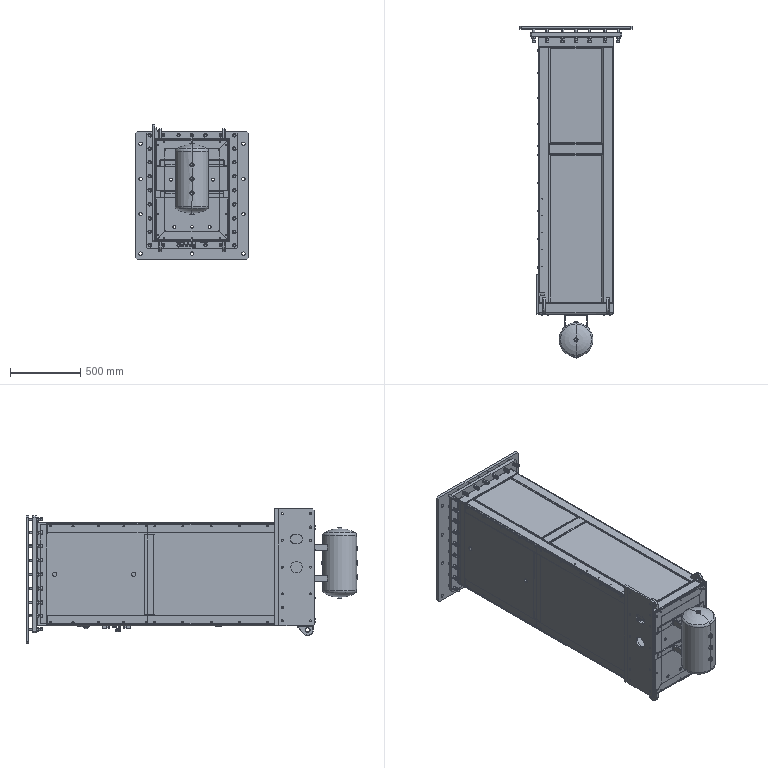Part | SolidWorks | features ReferencePattern 14, CompositeCurve 2, LocalLPattern 1 | 474 solids | 10459 faces | volume 70550722 mm3 | plane 4404 | cylinder 3811 | cone 1318 | torus 843 | spline 56 | sphere 27 | commonest cylinder face diameters 4.5 x474 4.1 x339 6.287 x339 4 x326 9 x250 3.3 x228